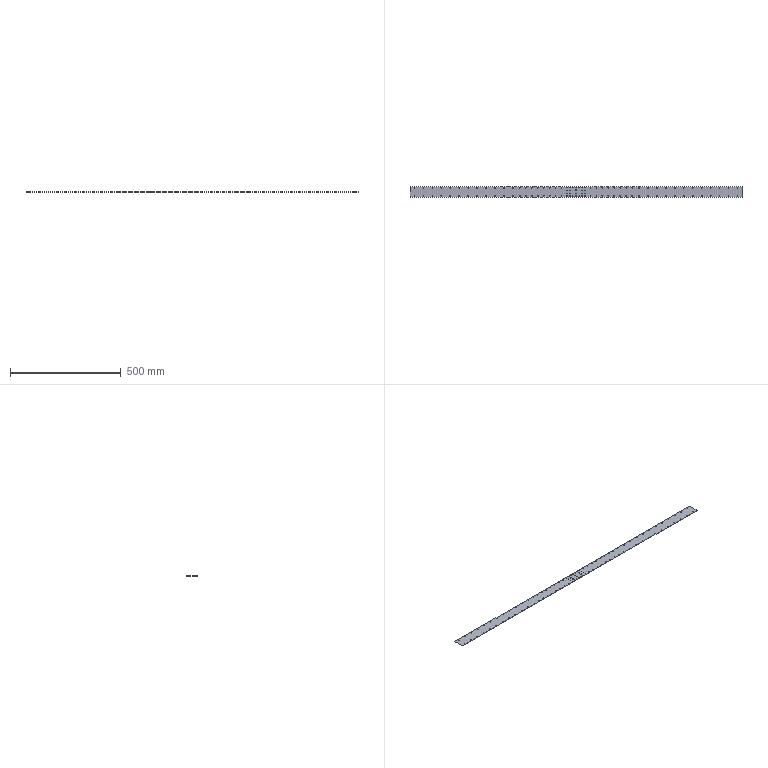Part | SolidWorks | features BaseBody 1 | 1 solid | 214 faces | box 1500 x 48 x 0.5 mm | volume 35620 mm3 | cylinder 208 | plane 6 | commonest cylinder face diameters 3.116 x96 3.2 x80 2.4 x32